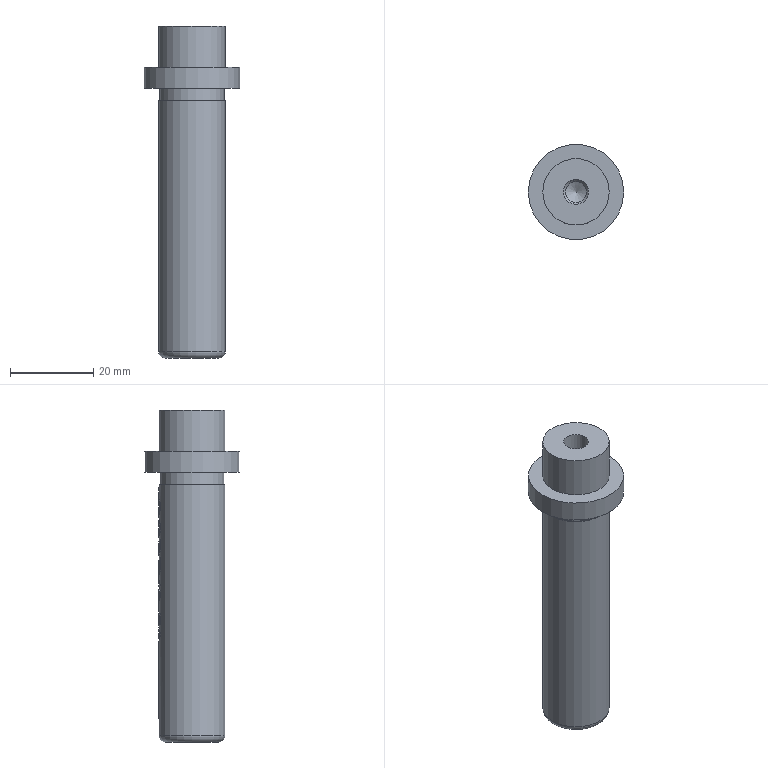Part | NX | features SGPR16-50_1 2 | 1 solid | 146 faces | box 23 x 23 x 80 mm | volume 16612 mm3 | plane 77 | cylinder 66 | cone 2 | torus 1 | commonest cylinder face diameters 15.8 x9 16 x6 1.458 x1 1.51 x1 1.734 x1 1.807 x1